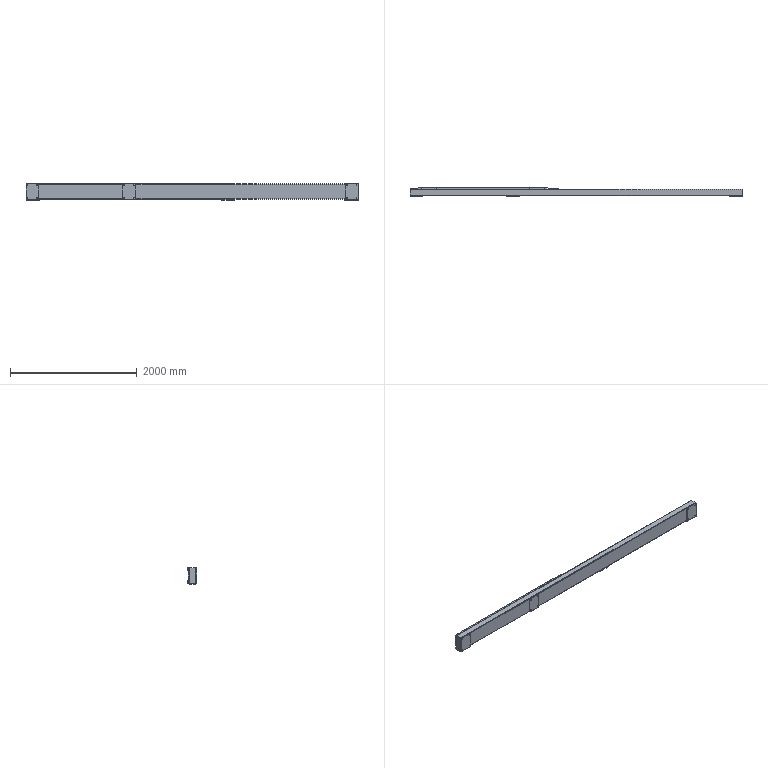Part | SolidWorks | features ICE 7, HoleWzd 6, Cut 1, DeleteBody 1, LPattern 1, MirrorSolid 1, WeldCornerFeat 1, WeldMemberFeat 1, WeldmentFeature 1 | 13 solids | 504 faces | box 5240 x 145 x 265 mm | volume 23826914 mm3 | cylinder 260 | cone 128 | plane 116 | commonest cylinder face diameters 6.8 x104 10.2 x88 8.5 x32 8 x12 2.5 x8 4.2 x8